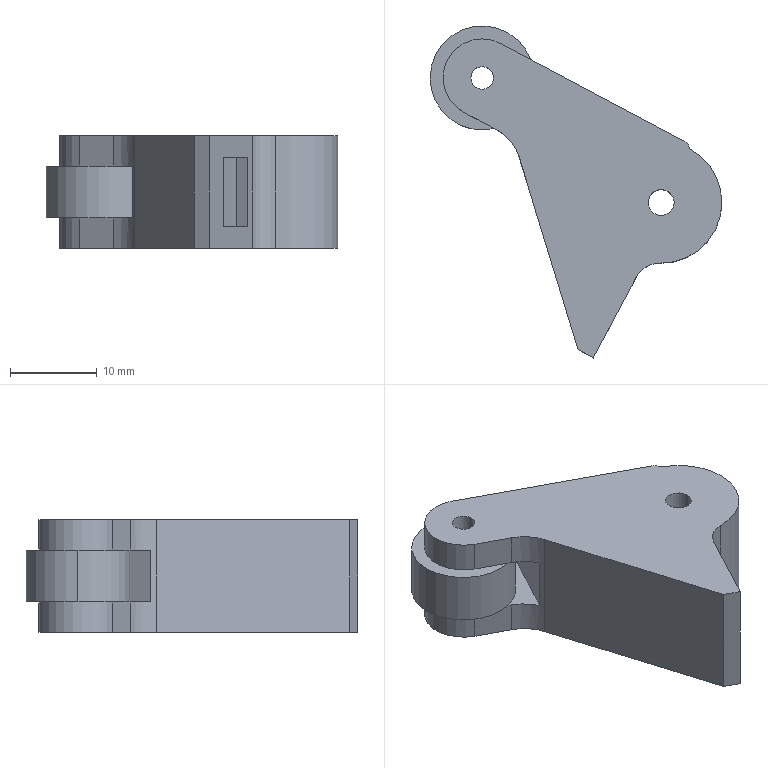Part | STEP file | 1105WWT3_1 | 1 solid | 33 faces | box 33.665 x 38.307 x 13 mm | volume 6665 mm3 | plane 19 | cylinder 14 | commonest cylinder face diameters 2.6 x2 3 x2 9 x2 12 x2 14 x2 1 x1
STEP:
#1=CARTESIAN_POINT('',(-37.5,12.,-6.5));
#2=VERTEX_POINT('',#1);
#3=CARTESIAN_POINT('',(-34.5,12.,-6.5));
#4=VERTEX_POINT('',#3);
#5=CARTESIAN_POINT('',(-36.,12.,-6.5));
#6=DIRECTION('',(0.,0.,1.));
#7=DIRECTION('',(1.,0.,0.));
#8=AXIS2_PLACEMENT_3D('',#5,#6,#7);
#9=CIRCLE('',#8,1.5);
#10=EDGE_CURVE('',#2,#4,#9,.T.);
#11=ORIENTED_EDGE('',*,*,#10,.F.);
#12=CARTESIAN_POINT('',(-37.5,12.,6.5));
#13=VERTEX_POINT('',#12);
#14=CARTESIAN_POINT('',(-37.5,12.,6.5));
#15=DIRECTION('',(0.,0.,1.));
#16=VECTOR('',#15,1000.);
#17=LINE('',#14,#16);
#18=EDGE_CURVE('',#2,#13,#17,.T.);
#19=ORIENTED_EDGE('',*,*,#18,.T.);
#20=CARTESIAN_POINT('',(-34.5,12.,6.5));
#21=VERTEX_POINT('',#20);
#22=CARTESIAN_POINT('',(-36.,12.,6.5));
#23=DIRECTION('',(0.,0.,-1.));
#24=DIRECTION('',(1.,0.,0.));
#25=AXIS2_PLACEMENT_3D('',#22,#23,#24);
#26=CIRCLE('',#25,1.5);
#27=EDGE_CURVE('',#21,#13,#26,.T.);
#28=ORIENTED_EDGE('',*,*,#27,.F.);
#29=CARTESIAN_POINT('',(-34.5,12.,6.5));
#30=DIRECTION('',(0.,0.,1.));
#31=VECTOR('',#30,1000.);
#32=LINE('',#29,#31);
#33=EDGE_CURVE('',#4,#21,#32,.T.);
#34=ORIENTED_EDGE('',*,*,#33,.F.);
#35=EDGE_LOOP('',(#11,#19,#28,#34));
#36=FACE_OUTER_BOUND('',#35,.T.);
#37=CARTESIAN_POINT('',(-36.,12.,6.5));
#38=DIRECTION('',(0.,0.,1.));
#39=DIRECTION('',(1.,0.,0.));
#40=AXIS2_PLACEMENT_3D('',#37,#38,#39);
#41=CYLINDRICAL_SURFACE('',#40,1.5);
#42=ADVANCED_FACE('',(#36),#41,.F.);
#43=CARTESIAN_POINT('',(-57.965,26.386,-6.5));
#44=VERTEX_POINT('',#43);
#45=CARTESIAN_POINT('',(-55.365,26.386,-6.5));
#46=VERTEX_POINT('',#45);
#47=CARTESIAN_POINT('',(-56.665,26.386,-6.5));
#48=DIRECTION('',(0.,0.,1.));
#49=DIRECTION('',(1.,0.,0.));
#50=AXIS2_PLACEMENT_3D('',#47,#48,#49);
#51=CIRCLE('',#50,1.3);
#52=EDGE_CURVE('',#44,#46,#51,.T.);
#53=ORIENTED_EDGE('',*,*,#52,.F.);
#54=CARTESIAN_POINT('',(-57.965,26.386,6.5));
#55=VERTEX_POINT('',#54);
#56=CARTESIAN_POINT('',(-57.965,26.386,6.5));
#57=DIRECTION('',(0.,0.,1.));
#58=VECTOR('',#57,1000.);
#59=LINE('',#56,#58);
#60=EDGE_CURVE('',#44,#55,#59,.T.);
#61=ORIENTED_EDGE('',*,*,#60,.T.);
#62=CARTESIAN_POINT('',(-55.365,26.386,6.5));
#63=VERTEX_POINT('',#62);
#64=CARTESIAN_POINT('',(-56.665,26.386,6.5));
#65=DIRECTION('',(0.,0.,-1.));
#66=DIRECTION('',(1.,0.,0.));
#67=AXIS2_PLACEMENT_3D('',#64,#65,#66);
#68=CIRCLE('',#67,1.3);
#69=EDGE_CURVE('',#63,#55,#68,.T.);
#70=ORIENTED_EDGE('',*,*,#69,.F.);
#71=CARTESIAN_POINT('',(-55.365,26.386,6.5));
#72=DIRECTION('',(0.,0.,1.));
#73=VECTOR('',#72,1000.);
#74=LINE('',#71,#73);
#75=EDGE_CURVE('',#46,#63,#74,.T.);
#76=ORIENTED_EDGE('',*,*,#75,.F.);
#77=EDGE_LOOP('',(#53,#61,#70,#76));
#78=FACE_OUTER_BOUND('',#77,.T.);
#79=CARTESIAN_POINT('',(-56.665,26.386,6.5));
#80=DIRECTION('',(0.,0.,1.));
#81=DIRECTION('',(1.,0.,0.));
#82=AXIS2_PLACEMENT_3D('',#79,#80,#81);
#83=CYLINDRICAL_SURFACE('',#82,1.3);
#84=ADVANCED_FACE('',(#78),#83,.F.);
#85=CARTESIAN_POINT('',(-36.153,5.002,-6.5));
#86=VERTEX_POINT('',#85);
#87=CARTESIAN_POINT('',(-29.,12.,-6.5));
#88=VERTEX_POINT('',#87);
#89=CARTESIAN_POINT('',(-36.,12.,-6.5));
#90=DIRECTION('',(0.,0.,1.));
#91=DIRECTION('',(1.,0.,0.));
#92=AXIS2_PLACEMENT_3D('',#89,#90,#91);
#93=CIRCLE('',#92,7.);
#94=EDGE_CURVE('',#86,#88,#93,.T.);
#95=ORIENTED_EDGE('',*,*,#94,.T.);
#96=CARTESIAN_POINT('',(-29.,12.,6.5));
#97=VERTEX_POINT('',#96);
#98=CARTESIAN_POINT('',(-29.,12.,6.5));
#99=DIRECTION('',(0.,0.,1.));
#100=VECTOR('',#99,1000.);
#101=LINE('',#98,#100);
#102=EDGE_CURVE('',#88,#97,#101,.T.);
#103=ORIENTED_EDGE('',*,*,#102,.T.);
#104=CARTESIAN_POINT('',(-36.153,5.002,6.5));
#105=VERTEX_POINT('',#104);
#106=CARTESIAN_POINT('',(-36.,12.,6.5));
#107=DIRECTION('',(0.,0.,1.));
#108=DIRECTION('',(1.,0.,0.));
#109=AXIS2_PLACEMENT_3D('',#106,#107,#108);
#110=CIRCLE('',#109,7.);
#111=EDGE_CURVE('',#105,#97,#110,.T.);
#112=ORIENTED_EDGE('',*,*,#111,.F.);
#113=CARTESIAN_POINT('',(-36.153,5.002,6.5));
#114=DIRECTION('',(0.,0.,-1.));
#115=VECTOR('',#114,1000.);
#116=LINE('',#113,#115);
#117=EDGE_CURVE('',#105,#86,#116,.T.);
#118=ORIENTED_EDGE('',*,*,#117,.T.);
#119=EDGE_LOOP('',(#95,#103,#112,#118));
#120=FACE_OUTER_BOUND('',#119,.T.);
#121=CARTESIAN_POINT('',(-36.,12.,6.5));
#122=DIRECTION('',(0.,0.,1.));
#123=DIRECTION('',(1.,0.,0.));
#124=AXIS2_PLACEMENT_3D('',#121,#122,#123);
#125=CYLINDRICAL_SURFACE('',#124,7.);
#126=ADVANCED_FACE('',(#120),#125,.T.);
#127=CARTESIAN_POINT('',(-51.049,28.496,-3.));
#128=VERTEX_POINT('',#127);
#129=CARTESIAN_POINT('',(-62.665,26.386,-3.));
#130=VERTEX_POINT('',#129);
#131=CARTESIAN_POINT('',(-56.665,26.386,-3.));
#132=DIRECTION('',(0.,0.,1.));
#133=DIRECTION('',(1.,0.,0.));
#134=AXIS2_PLACEMENT_3D('',#131,#132,#133);
#135=CIRCLE('',#134,6.);
#136=EDGE_CURVE('',#128,#130,#135,.T.);
#137=ORIENTED_EDGE('',*,*,#136,.T.);
#138=CARTESIAN_POINT('',(-62.665,26.386,3.));
#139=VERTEX_POINT('',#138);
#140=CARTESIAN_POINT('',(-62.665,26.386,3.));
#141=DIRECTION('',(0.,0.,1.));
#142=VECTOR('',#141,1000.);
#143=LINE('',#140,#142);
#144=EDGE_CURVE('',#130,#139,#143,.T.);
#145=ORIENTED_EDGE('',*,*,#144,.T.);
#146=CARTESIAN_POINT('',(-51.049,28.496,3.));
#147=VERTEX_POINT('',#146);
#148=CARTESIAN_POINT('',(-56.665,26.386,3.));
#149=DIRECTION('',(0.,0.,1.));
#150=DIRECTION('',(1.,0.,0.));
#151=AXIS2_PLACEMENT_3D('',#148,#149,#150);
#152=CIRCLE('',#151,6.);
#153=EDGE_CURVE('',#147,#139,#152,.T.);
#154=ORIENTED_EDGE('',*,*,#153,.F.);
#155=CARTESIAN_POINT('',(-50.665,26.386,3.));
#156=VERTEX_POINT('',#155);
#157=CARTESIAN_POINT('',(-56.665,26.386,3.));
#158=DIRECTION('',(0.,0.,-1.));
#159=DIRECTION('',(1.,0.,0.));
#160=AXIS2_PLACEMENT_3D('',#157,#158,#159);
#161=CIRCLE('',#160,6.);
#162=EDGE_CURVE('',#147,#156,#161,.T.);
#163=ORIENTED_EDGE('',*,*,#162,.T.);
#164=CARTESIAN_POINT('',(-50.665,26.386,-3.));
#165=VERTEX_POINT('',#164);
#166=CARTESIAN_POINT('',(-50.665,26.386,3.));
#167=DIRECTION('',(0.,0.,1.));
#168=VECTOR('',#167,1000.);
#169=LINE('',#166,#168);
#170=EDGE_CURVE('',#165,#156,#169,.T.);
#171=ORIENTED_EDGE('',*,*,#170,.F.);
#172=CARTESIAN_POINT('',(-56.665,26.386,-3.));
#173=DIRECTION('',(0.,0.,-1.));
#174=DIRECTION('',(1.,0.,0.));
#175=AXIS2_PLACEMENT_3D('',#172,#173,#174);
#176=CIRCLE('',#175,6.);
#177=EDGE_CURVE('',#128,#165,#176,.T.);
#178=ORIENTED_EDGE('',*,*,#177,.F.);
#179=EDGE_LOOP('',(#137,#145,#154,#163,#171,#178));
#180=FACE_OUTER_BOUND('',#179,.T.);
#181=CARTESIAN_POINT('',(-56.665,26.386,3.));
#182=DIRECTION('',(0.,0.,1.));
#183=DIRECTION('',(1.,0.,0.));
#184=AXIS2_PLACEMENT_3D('',#181,#182,#183);
#185=CYLINDRICAL_SURFACE('',#184,6.);
#186=ADVANCED_FACE('',(#180),#185,.T.);
#187=ORIENTED_EDGE('',*,*,#27,.T.);
#188=CARTESIAN_POINT('',(-36.,12.,6.5));
#189=DIRECTION('',(0.,0.,-1.));
#190=DIRECTION('',(1.,0.,0.));
#191=AXIS2_PLACEMENT_3D('',#188,#189,#190);
#192=CIRCLE('',#191,1.5);
#193=EDGE_CURVE('',#13,#21,#192,.T.);
#194=ORIENTED_EDGE('',*,*,#193,.T.);
#195=EDGE_LOOP('',(#187,#194));
#196=FACE_BOUND('',#195,.T.);
#197=ORIENTED_EDGE('',*,*,#69,.T.);
#198=CARTESIAN_POINT('',(-56.665,26.386,6.5));
#199=DIRECTION('',(0.,0.,-1.));
#200=DIRECTION('',(1.,0.,0.));
#201=AXIS2_PLACEMENT_3D('',#198,#199,#200);
#202=CIRCLE('',#201,1.3);
#203=EDGE_CURVE('',#55,#63,#202,.T.);
#204=ORIENTED_EDGE('',*,*,#203,.T.);
#205=EDGE_LOOP('',(#197,#204));
#206=FACE_BOUND('',#205,.T.);
#207=CARTESIAN_POINT('',(-52.433,17.38,6.5));
#208=VERTEX_POINT('',#207);
#209=CARTESIAN_POINT('',(-45.596,-4.983,6.5));
#210=VERTEX_POINT('',#209);
#211=CARTESIAN_POINT('',(-52.433,17.38,6.5));
#212=DIRECTION('',(0.2924,-0.9563,0.));
#213=VECTOR('',#212,1000.);
#214=LINE('',#211,#213);
#215=EDGE_CURVE('',#208,#210,#214,.T.);
#216=ORIENTED_EDGE('',*,*,#215,.T.);
#217=CARTESIAN_POINT('',(-43.83,-5.922,6.5));
#218=VERTEX_POINT('',#217);
#219=CARTESIAN_POINT('',(-45.596,-4.983,6.5));
#220=DIRECTION('',(0.8829,-0.4695,0.));
#221=VECTOR('',#220,1000.);
#222=LINE('',#219,#221);
#223=EDGE_CURVE('',#210,#218,#222,.T.);
#224=ORIENTED_EDGE('',*,*,#223,.T.);
#225=CARTESIAN_POINT('',(-38.868,3.411,6.5));
#226=VERTEX_POINT('',#225);
#227=CARTESIAN_POINT('',(-43.83,-5.922,6.5));
#228=DIRECTION('',(0.4695,0.8829,0.));
#229=VECTOR('',#228,1000.);
#230=LINE('',#227,#229);
#231=EDGE_CURVE('',#218,#226,#230,.T.);
#232=ORIENTED_EDGE('',*,*,#231,.T.);
#233=CARTESIAN_POINT('',(-36.219,2.002,6.5));
#234=DIRECTION('',(0.,0.,-1.));
#235=DIRECTION('',(1.,0.,0.));
#236=AXIS2_PLACEMENT_3D('',#233,#234,#235);
#237=CIRCLE('',#236,3.);
#238=EDGE_CURVE('',#226,#105,#237,.T.);
#239=ORIENTED_EDGE('',*,*,#238,.T.);
#240=ORIENTED_EDGE('',*,*,#111,.T.);
#241=CARTESIAN_POINT('',(-32.542,18.086,6.5));
#242=VERTEX_POINT('',#241);
#243=CARTESIAN_POINT('',(-36.,12.,6.5));
#244=DIRECTION('',(0.,0.,1.));
#245=DIRECTION('',(1.,0.,0.));
#246=AXIS2_PLACEMENT_3D('',#243,#244,#245);
#247=CIRCLE('',#246,7.);
#248=EDGE_CURVE('',#97,#242,#247,.T.);
#249=ORIENTED_EDGE('',*,*,#248,.T.);
#250=CARTESIAN_POINT('',(-32.773,18.375,6.5));
#251=VERTEX_POINT('',#250);
#252=CARTESIAN_POINT('',(-32.295,18.521,6.5));
#253=DIRECTION('',(0.,0.,-1.));
#254=DIRECTION('',(1.,0.,0.));
#255=AXIS2_PLACEMENT_3D('',#252,#253,#254);
#256=CIRCLE('',#255,0.5);
#257=EDGE_CURVE('',#242,#251,#256,.T.);
#258=ORIENTED_EDGE('',*,*,#257,.T.);
#259=CARTESIAN_POINT('',(-32.799,18.461,6.5));
#260=VERTEX_POINT('',#259);
#261=CARTESIAN_POINT('',(-32.773,18.375,6.5));
#262=DIRECTION('',(0.2924,-0.9563,0.));
#263=VECTOR('',#262,1000.);
#264=LINE('',#261,#263);
#265=EDGE_CURVE('',#260,#251,#264,.T.);
#266=ORIENTED_EDGE('',*,*,#265,.F.);
#267=CARTESIAN_POINT('',(-33.286,19.051,6.5));
#268=VERTEX_POINT('',#267);
#269=CARTESIAN_POINT('',(-33.756,18.168,6.5));
#270=DIRECTION('',(0.,0.,-1.));
#271=DIRECTION('',(1.,0.,0.));
#272=AXIS2_PLACEMENT_3D('',#269,#270,#271);
#273=CIRCLE('',#272,1.);
#274=EDGE_CURVE('',#268,#260,#273,.T.);
#275=ORIENTED_EDGE('',*,*,#274,.F.);
#276=CARTESIAN_POINT('',(-54.553,30.359,6.5));
#277=VERTEX_POINT('',#276);
#278=CARTESIAN_POINT('',(-33.286,19.051,6.5));
#279=DIRECTION('',(-0.8829,0.4695,0.));
#280=VECTOR('',#279,1000.);
#281=LINE('',#278,#280);
#282=EDGE_CURVE('',#268,#277,#281,.T.);
#283=ORIENTED_EDGE('',*,*,#282,.T.);
#284=CARTESIAN_POINT('',(-58.778,22.412,6.5));
#285=VERTEX_POINT('',#284);
#286=CARTESIAN_POINT('',(-56.665,26.386,6.5));
#287=DIRECTION('',(0.,0.,1.));
#288=DIRECTION('',(1.,0.,0.));
#289=AXIS2_PLACEMENT_3D('',#286,#287,#288);
#290=CIRCLE('',#289,4.5);
#291=EDGE_CURVE('',#277,#285,#290,.T.);
#292=ORIENTED_EDGE('',*,*,#291,.T.);
#293=CARTESIAN_POINT('',(-54.867,20.333,6.5));
#294=VERTEX_POINT('',#293);
#295=CARTESIAN_POINT('',(-58.778,22.412,6.5));
#296=DIRECTION('',(0.8829,-0.4695,0.));
#297=VECTOR('',#296,1000.);
#298=LINE('',#295,#297);
#299=EDGE_CURVE('',#285,#294,#298,.T.);
#300=ORIENTED_EDGE('',*,*,#299,.T.);
#301=CARTESIAN_POINT('',(-57.215,15.918,6.5));
#302=DIRECTION('',(0.,0.,-1.));
#303=DIRECTION('',(1.,0.,0.));
#304=AXIS2_PLACEMENT_3D('',#301,#302,#303);
#305=CIRCLE('',#304,5.);
#306=EDGE_CURVE('',#294,#208,#305,.T.);
#307=ORIENTED_EDGE('',*,*,#306,.T.);
#308=EDGE_LOOP('',(#216,#224,#232,#239,#240,#249,#258,#266,#275,#283,#292,#300,#307));
#309=FACE_OUTER_BOUND('',#308,.T.);
#310=CARTESIAN_POINT('',(-36.,12.,6.5));
#311=DIRECTION('',(0.,0.,1.));
#312=DIRECTION('',(1.,0.,0.));
#313=AXIS2_PLACEMENT_3D('',#310,#311,#312);
#314=PLANE('',#313);
#315=ADVANCED_FACE('',(#196,#206,#309),#314,.T.);
#316=ORIENTED_EDGE('',*,*,#18,.F.);
#317=CARTESIAN_POINT('',(-36.,12.,-6.5));
#318=DIRECTION('',(0.,0.,1.));
#319=DIRECTION('',(1.,0.,0.));
#320=AXIS2_PLACEMENT_3D('',#317,#318,#319);
#321=CIRCLE('',#320,1.5);
#322=EDGE_CURVE('',#4,#2,#321,.T.);
#323=ORIENTED_EDGE('',*,*,#322,.F.);
#324=ORIENTED_EDGE('',*,*,#33,.T.);
#325=ORIENTED_EDGE('',*,*,#193,.F.);
#326=EDGE_LOOP('',(#316,#323,#324,#325));
#327=FACE_OUTER_BOUND('',#326,.T.);
#328=CARTESIAN_POINT('',(-36.,12.,6.5));
#329=DIRECTION('',(0.,0.,1.));
#330=DIRECTION('',(1.,0.,0.));
#331=AXIS2_PLACEMENT_3D('',#328,#329,#330);
#332=CYLINDRICAL_SURFACE('',#331,1.5);
#333=ADVANCED_FACE('',(#327),#332,.F.);
#334=ORIENTED_EDGE('',*,*,#60,.F.);
#335=CARTESIAN_POINT('',(-56.665,26.386,-6.5));
#336=DIRECTION('',(0.,0.,1.));
#337=DIRECTION('',(1.,0.,0.));
#338=AXIS2_PLACEMENT_3D('',#335,#336,#337);
#339=CIRCLE('',#338,1.3);
#340=EDGE_CURVE('',#46,#44,#339,.T.);
#341=ORIENTED_EDGE('',*,*,#340,.F.);
#342=ORIENTED_EDGE('',*,*,#75,.T.);
#343=ORIENTED_EDGE('',*,*,#203,.F.);
#344=EDGE_LOOP('',(#334,#341,#342,#343));
#345=FACE_OUTER_BOUND('',#344,.T.);
#346=CARTESIAN_POINT('',(-56.665,26.386,6.5));
#347=DIRECTION('',(0.,0.,1.));
#348=DIRECTION('',(1.,0.,0.));
#349=AXIS2_PLACEMENT_3D('',#346,#347,#348);
#350=CYLINDRICAL_SURFACE('',#349,1.3);
#351=ADVANCED_FACE('',(#345),#350,.F.);
#352=ORIENTED_EDGE('',*,*,#223,.F.);
#353=CARTESIAN_POINT('',(-45.596,-4.983,-6.5));
#354=VERTEX_POINT('',#353);
#355=CARTESIAN_POINT('',(-45.596,-4.983,6.5));
#356=DIRECTION('',(0.,0.,-1.));
#357=VECTOR('',#356,1000.);
#358=LINE('',#355,#357);
#359=EDGE_CURVE('',#210,#354,#358,.T.);
#360=ORIENTED_EDGE('',*,*,#359,.T.);
#361=CARTESIAN_POINT('',(-43.83,-5.922,-6.5));
#362=VERTEX_POINT('',#361);
#363=CARTESIAN_POINT('',(-45.596,-4.983,-6.5));
#364=DIRECTION('',(0.8829,-0.4695,0.));
#365=VECTOR('',#364,1000.);
#366=LINE('',#363,#365);
#367=EDGE_CURVE('',#354,#362,#366,.T.);
#368=ORIENTED_EDGE('',*,*,#367,.T.);
#369=CARTESIAN_POINT('',(-43.83,-5.922,6.5));
#370=DIRECTION('',(0.,0.,1.));
#371=VECTOR('',#370,1000.);
#372=LINE('',#369,#371);
#373=EDGE_CURVE('',#362,#218,#372,.T.);
#374=ORIENTED_EDGE('',*,*,#373,.T.);
#375=EDGE_LOOP('',(#352,#360,#368,#374));
#376=FACE_OUTER_BOUND('',#375,.T.);
#377=CARTESIAN_POINT('',(-45.596,-4.983,6.5));
#378=DIRECTION('',(-0.4695,-0.8829,0.));
#379=DIRECTION('',(0.8829,-0.4695,0.));
#380=AXIS2_PLACEMENT_3D('',#377,#378,#379);
#381=PLANE('',#380);
#382=ADVANCED_FACE('',(#376),#381,.T.);
#383=ORIENTED_EDGE('',*,*,#215,.F.);
#384=CARTESIAN_POINT('',(-52.433,17.38,-6.5));
#385=VERTEX_POINT('',#384);
#386=CARTESIAN_POINT('',(-52.433,17.38,6.5));
#387=DIRECTION('',(0.,0.,-1.));
#388=VECTOR('',#387,1000.);
#389=LINE('',#386,#388);
#390=EDGE_CURVE('',#208,#385,#389,.T.);
#391=ORIENTED_EDGE('',*,*,#390,.T.);
#392=CARTESIAN_POINT('',(-52.433,17.38,-6.5));
#393=DIRECTION('',(0.2924,-0.9563,0.));
#394=VECTOR('',#393,1000.);
#395=LINE('',#392,#394);
#396=EDGE_CURVE('',#385,#354,#395,.T.);
#397=ORIENTED_EDGE('',*,*,#396,.T.);
#398=ORIENTED_EDGE('',*,*,#359,.F.);
#399=EDGE_LOOP('',(#383,#391,#397,#398));
#400=FACE_OUTER_BOUND('',#399,.T.);
#401=CARTESIAN_POINT('',(-52.433,17.38,6.5));
#402=DIRECTION('',(-0.9563,-0.2924,0.));
#403=DIRECTION('',(0.2924,-0.9563,0.));
#404=AXIS2_PLACEMENT_3D('',#401,#402,#403);
#405=PLANE('',#404);
#406=ADVANCED_FACE('',(#400),#405,.T.);
#407=CARTESIAN_POINT('',(-54.867,20.333,-6.5));
#408=VERTEX_POINT('',#407);
#409=CARTESIAN_POINT('',(-54.867,20.333,-3.));
#410=VERTEX_POINT('',#409);
#411=CARTESIAN_POINT('',(-54.867,20.333,6.5));
#412=DIRECTION('',(0.,0.,1.));
#413=VECTOR('',#412,1000.);
#414=LINE('',#411,#413);
#415=EDGE_CURVE('',#408,#410,#414,.T.);
#416=ORIENTED_EDGE('',*,*,#415,.F.);
#417=CARTESIAN_POINT('',(-57.215,15.918,-6.5));
#418=DIRECTION('',(0.,0.,1.));
#419=DIRECTION('',(1.,0.,0.));
#420=AXIS2_PLACEMENT_3D('',#417,#418,#419);
#421=CIRCLE('',#420,5.);
#422=EDGE_CURVE('',#385,#408,#421,.T.);
#423=ORIENTED_EDGE('',*,*,#422,.F.);
#424=ORIENTED_EDGE('',*,*,#390,.F.);
#425=ORIENTED_EDGE('',*,*,#306,.F.);
#426=CARTESIAN_POINT('',(-54.867,20.333,3.));
#427=VERTEX_POINT('',#426);
#428=CARTESIAN_POINT('',(-54.867,20.333,6.5));
#429=DIRECTION('',(0.,0.,1.));
#430=VECTOR('',#429,1000.);
#431=LINE('',#428,#430);
#432=EDGE_CURVE('',#427,#294,#431,.T.);
#433=ORIENTED_EDGE('',*,*,#432,.F.);
#434=CARTESIAN_POINT('',(-52.651,17.96,3.));
#435=VERTEX_POINT('',#434);
#436=CARTESIAN_POINT('',(-57.215,15.918,3.));
#437=DIRECTION('',(0.,0.,1.));
#438=DIRECTION('',(1.,0.,0.));
#439=AXIS2_PLACEMENT_3D('',#436,#437,#438);
#440=CIRCLE('',#439,5.);
#441=EDGE_CURVE('',#435,#427,#440,.T.);
#442=ORIENTED_EDGE('',*,*,#441,.F.);
#443=CARTESIAN_POINT('',(-52.651,17.96,-3.));
#444=VERTEX_POINT('',#443);
#445=CARTESIAN_POINT('',(-52.651,17.96,6.5));
#446=DIRECTION('',(0.,0.,1.));
#447=VECTOR('',#446,1000.);
#448=LINE('',#445,#447);
#449=EDGE_CURVE('',#444,#435,#448,.T.);
#450=ORIENTED_EDGE('',*,*,#449,.F.);
#451=CARTESIAN_POINT('',(-57.215,15.918,-3.));
#452=DIRECTION('',(0.,0.,-1.));
#453=DIRECTION('',(1.,0.,0.));
#454=AXIS2_PLACEMENT_3D('',#451,#452,#453);
#455=CIRCLE('',#454,5.);
#456=EDGE_CURVE('',#410,#444,#455,.T.);
#457=ORIENTED_EDGE('',*,*,#456,.F.);
#458=EDGE_LOOP('',(#416,#423,#424,#425,#433,#442,#450,#457));
#459=FACE_OUTER_BOUND('',#458,.T.);
#460=CARTESIAN_POINT('',(-57.215,15.918,6.5));
#461=DIRECTION('',(0.,0.,1.));
#462=DIRECTION('',(1.,0.,0.));
#463=AXIS2_PLACEMENT_3D('',#460,#461,#462);
#464=CYLINDRICAL_SURFACE('',#463,5.);
#465=ADVANCED_FACE('',(#459),#464,.F.);
#466=ORIENTED_EDGE('',*,*,#299,.F.);
#467=CARTESIAN_POINT('',(-58.778,22.412,3.));
#468=VERTEX_POINT('',#467);
#469=CARTESIAN_POINT('',(-58.778,22.412,6.5));
#470=DIRECTION('',(0.,0.,-1.));
#471=VECTOR('',#470,1000.);
#472=LINE('',#469,#471);
#473=EDGE_CURVE('',#285,#468,#472,.T.);
#474=ORIENTED_EDGE('',*,*,#473,.T.);
#475=CARTESIAN_POINT('',(-55.274,20.549,3.));
#476=VERTEX_POINT('',#475);
#477=CARTESIAN_POINT('',(-58.778,22.412,3.));
#478=DIRECTION('',(0.8829,-0.4695,0.));
#479=VECTOR('',#478,1000.);
#480=LINE('',#477,#479);
#481=EDGE_CURVE('',#468,#476,#480,.T.);
#482=ORIENTED_EDGE('',*,*,#481,.T.);
#483=CARTESIAN_POINT('',(-58.778,22.412,3.));
#484=DIRECTION('',(0.8829,-0.4695,0.));
#485=VECTOR('',#484,1000.);
#486=LINE('',#483,#485);
#487=EDGE_CURVE('',#476,#427,#486,.T.);
#488=ORIENTED_EDGE('',*,*,#487,.T.);
#489=ORIENTED_EDGE('',*,*,#432,.T.);
#490=EDGE_LOOP('',(#466,#474,#482,#488,#489));
#491=FACE_OUTER_BOUND('',#490,.T.);
#492=CARTESIAN_POINT('',(-58.778,22.412,6.5));
#493=DIRECTION('',(-0.4695,-0.8829,0.));
#494=DIRECTION('',(0.8829,-0.4695,0.));
#495=AXIS2_PLACEMENT_3D('',#492,#493,#494);
#496=PLANE('',#495);
#497=ADVANCED_FACE('',(#491),#496,.T.);
#498=ORIENTED_EDGE('',*,*,#291,.F.);
#499=CARTESIAN_POINT('',(-54.553,30.359,3.));
#500=VERTEX_POINT('',#499);
#501=CARTESIAN_POINT('',(-54.553,30.359,6.5));
#502=DIRECTION('',(0.,0.,-1.));
#503=VECTOR('',#502,1000.);
#504=LINE('',#501,#503);
#505=EDGE_CURVE('',#277,#500,#504,.T.);
#506=ORIENTED_EDGE('',*,*,#505,.T.);
#507=CARTESIAN_POINT('',(-56.665,26.386,3.));
#508=DIRECTION('',(0.,0.,1.));
#509=DIRECTION('',(1.,0.,0.));
#510=AXIS2_PLACEMENT_3D('',#507,#508,#509);
#511=CIRCLE('',#510,4.5);
#512=EDGE_CURVE('',#500,#468,#511,.T.);
#513=ORIENTED_EDGE('',*,*,#512,.T.);
#514=ORIENTED_EDGE('',*,*,#473,.F.);
#515=EDGE_LOOP('',(#498,#506,#513,#514));
#516=FACE_OUTER_BOUND('',#515,.T.);
#517=CARTESIAN_POINT('',(-56.665,26.386,6.5));
#518=DIRECTION('',(0.,0.,1.));
#519=DIRECTION('',(1.,0.,0.));
#520=AXIS2_PLACEMENT_3D('',#517,#518,#519);
#521=CYLINDRICAL_SURFACE('',#520,4.5);
#522=ADVANCED_FACE('',(#516),#521,.T.);
#523=CARTESIAN_POINT('',(-33.286,19.051,-6.5));
#524=VERTEX_POINT('',#523);
#525=CARTESIAN_POINT('',(-54.553,30.359,-6.5));
#526=VERTEX_POINT('',#525);
#527=CARTESIAN_POINT('',(-33.286,19.051,-6.5));
#528=DIRECTION('',(-0.8829,0.4695,0.));
#529=VECTOR('',#528,1000.);
#530=LINE('',#527,#529);
#531=EDGE_CURVE('',#524,#526,#530,.T.);
#532=ORIENTED_EDGE('',*,*,#531,.T.);
#533=CARTESIAN_POINT('',(-54.553,30.359,-3.));
#534=VERTEX_POINT('',#533);
#535=CARTESIAN_POINT('',(-54.553,30.359,6.5));
#536=DIRECTION('',(0.,0.,1.));
#537=VECTOR('',#536,1000.);
#538=LINE('',#535,#537);
#539=EDGE_CURVE('',#526,#534,#538,.T.);
#540=ORIENTED_EDGE('',*,*,#539,.T.);
#541=CARTESIAN_POINT('',(-33.286,19.051,-3.));
#542=DIRECTION('',(0.8829,-0.4695,0.));
#543=VECTOR('',#542,1000.);
#544=LINE('',#541,#543);
#545=EDGE_CURVE('',#534,#128,#544,.T.);
#546=ORIENTED_EDGE('',*,*,#545,.T.);
#547=CARTESIAN_POINT('',(-47.931,26.838,-3.));
#548=VERTEX_POINT('',#547);
#549=CARTESIAN_POINT('',(-33.286,19.051,-3.));
#550=DIRECTION('',(0.8829,-0.4695,0.));
#551=VECTOR('',#550,1000.);
#552=LINE('',#549,#551);
#553=EDGE_CURVE('',#128,#548,#552,.T.);
#554=ORIENTED_EDGE('',*,*,#553,.T.);
#555=CARTESIAN_POINT('',(-47.931,26.838,3.));
#556=VERTEX_POINT('',#555);
#557=CARTESIAN_POINT('',(-47.931,26.838,6.5));
#558=DIRECTION('',(0.,0.,1.));
#559=VECTOR('',#558,1000.);
#560=LINE('',#557,#559);
#561=EDGE_CURVE('',#548,#556,#560,.T.);
#562=ORIENTED_EDGE('',*,*,#561,.T.);
#563=CARTESIAN_POINT('',(-33.286,19.051,3.));
#564=DIRECTION('',(-0.8829,0.4695,0.));
#565=VECTOR('',#564,1000.);
#566=LINE('',#563,#565);
#567=EDGE_CURVE('',#556,#147,#566,.T.);
#568=ORIENTED_EDGE('',*,*,#567,.T.);
#569=CARTESIAN_POINT('',(-33.286,19.051,3.));
#570=DIRECTION('',(-0.8829,0.4695,0.));
#571=VECTOR('',#570,1000.);
#572=LINE('',#569,#571);
#573=EDGE_CURVE('',#147,#500,#572,.T.);
#574=ORIENTED_EDGE('',*,*,#573,.T.);
#575=ORIENTED_EDGE('',*,*,#505,.F.);
#576=ORIENTED_EDGE('',*,*,#282,.F.);
#577=CARTESIAN_POINT('',(-33.286,19.051,6.5));
#578=DIRECTION('',(0.,0.,-1.));
#579=VECTOR('',#578,1000.);
#580=LINE('',#577,#579);
#581=EDGE_CURVE('',#268,#524,#580,.T.);
#582=ORIENTED_EDGE('',*,*,#581,.T.);
#583=EDGE_LOOP('',(#532,#540,#546,#554,#562,#568,#574,#575,#576,#582));
#584=FACE_OUTER_BOUND('',#583,.T.);
#585=CARTESIAN_POINT('',(-33.286,19.051,6.5));
#586=DIRECTION('',(0.4695,0.8829,0.));
#587=DIRECTION('',(-0.8829,0.4695,0.));
#588=AXIS2_PLACEMENT_3D('',#585,#586,#587);
#589=PLANE('',#588);
#590=ADVANCED_FACE('',(#584),#589,.T.);
#591=ORIENTED_EDGE('',*,*,#102,.F.);
#592=CARTESIAN_POINT('',(-32.542,18.086,-6.5));
#593=VERTEX_POINT('',#592);
#594=CARTESIAN_POINT('',(-36.,12.,-6.5));
#595=DIRECTION('',(0.,0.,1.));
#596=DIRECTION('',(1.,0.,0.));
#597=AXIS2_PLACEMENT_3D('',#594,#595,#596);
#598=CIRCLE('',#597,7.);
#599=EDGE_CURVE('',#88,#593,#598,.T.);
#600=ORIENTED_EDGE('',*,*,#599,.T.);
#601=CARTESIAN_POINT('',(-32.542,18.086,6.5));
#602=DIRECTION('',(0.,0.,1.));
#603=VECTOR('',#602,1000.);
#604=LINE('',#601,#603);
#605=EDGE_CURVE('',#593,#242,#604,.T.);
#606=ORIENTED_EDGE('',*,*,#605,.T.);
#607=ORIENTED_EDGE('',*,*,#248,.F.);
#608=EDGE_LOOP('',(#591,#600,#606,#607));
#609=FACE_OUTER_BOUND('',#608,.T.);
#610=CARTESIAN_POINT('',(-36.,12.,6.5));
#611=DIRECTION('',(0.,0.,1.));
#612=DIRECTION('',(1.,0.,0.));
#613=AXIS2_PLACEMENT_3D('',#610,#611,#612);
#614=CYLINDRICAL_SURFACE('',#613,7.);
#615=ADVANCED_FACE('',(#609),#614,.T.);
#616=ORIENTED_EDGE('',*,*,#117,.F.);
#617=ORIENTED_EDGE('',*,*,#238,.F.);
#618=CARTESIAN_POINT('',(-38.868,3.411,-6.5));
#619=VERTEX_POINT('',#618);
#620=CARTESIAN_POINT('',(-38.868,3.411,6.5));
#621=DIRECTION('',(0.,0.,1.));
#622=VECTOR('',#621,1000.);
#623=LINE('',#620,#622);
#624=EDGE_CURVE('',#619,#226,#623,.T.);
#625=ORIENTED_EDGE('',*,*,#624,.F.);
#626=CARTESIAN_POINT('',(-36.219,2.002,-6.5));
#627=DIRECTION('',(0.,0.,1.));
#628=DIRECTION('',(1.,0.,0.));
#629=AXIS2_PLACEMENT_3D('',#626,#627,#628);
#630=CIRCLE('',#629,3.);
#631=EDGE_CURVE('',#86,#619,#630,.T.);
#632=ORIENTED_EDGE('',*,*,#631,.F.);
#633=EDGE_LOOP('',(#616,#617,#625,#632));
#634=FACE_OUTER_BOUND('',#633,.T.);
#635=CARTESIAN_POINT('',(-36.219,2.002,6.5));
#636=DIRECTION('',(0.,0.,1.));
#637=DIRECTION('',(1.,0.,0.));
#638=AXIS2_PLACEMENT_3D('',#635,#636,#637);
#639=CYLINDRICAL_SURFACE('',#638,3.);
#640=ADVANCED_FACE('',(#634),#639,.F.);
#641=ORIENTED_EDGE('',*,*,#231,.F.);
#642=ORIENTED_EDGE('',*,*,#373,.F.);
#643=CARTESIAN_POINT('',(-43.83,-5.922,-6.5));
#644=DIRECTION('',(0.4695,0.8829,0.));
#645=VECTOR('',#644,1000.);
#646=LINE('',#643,#645);
#647=EDGE_CURVE('',#362,#619,#646,.T.);
#648=ORIENTED_EDGE('',*,*,#647,.T.);
#649=ORIENTED_EDGE('',*,*,#624,.T.);
#650=EDGE_LOOP('',(#641,#642,#648,#649));
#651=FACE_OUTER_BOUND('',#650,.T.);
#652=CARTESIAN_POINT('',(-39.37,2.466,4.));
#653=VERTEX_POINT('',#652);
#654=CARTESIAN_POINT('',(-39.37,2.466,-4.));
#655=VERTEX_POINT('',#654);
#656=CARTESIAN_POINT('',(-39.37,2.466,6.5));
#657=DIRECTION('',(0.,0.,-1.));
#658=VECTOR('',#657,1000.);
#659=LINE('',#656,#658);
#660=EDGE_CURVE('',#653,#655,#659,.T.);
#661=ORIENTED_EDGE('',*,*,#660,.T.);
#662=CARTESIAN_POINT('',(-42.187,-2.831,-4.));
#663=VERTEX_POINT('',#662);
#664=CARTESIAN_POINT('',(-43.83,-5.922,-4.));
#665=DIRECTION('',(-0.4695,-0.8829,0.));
#666=VECTOR('',#665,1000.);
#667=LINE('',#664,#666);
#668=EDGE_CURVE('',#655,#663,#667,.T.);
#669=ORIENTED_EDGE('',*,*,#668,.T.);
#670=CARTESIAN_POINT('',(-42.187,-2.831,4.));
#671=VERTEX_POINT('',#670);
#672=CARTESIAN_POINT('',(-42.187,-2.831,6.5));
#673=DIRECTION('',(0.,0.,1.));
#674=VECTOR('',#673,1000.);
#675=LINE('',#672,#674);
#676=EDGE_CURVE('',#663,#671,#675,.T.);
#677=ORIENTED_EDGE('',*,*,#676,.T.);
#678=CARTESIAN_POINT('',(-43.83,-5.922,4.));
#679=DIRECTION('',(0.4695,0.8829,0.));
#680=VECTOR('',#679,1000.);
#681=LINE('',#678,#680);
#682=EDGE_CURVE('',#671,#653,#681,.T.);
#683=ORIENTED_EDGE('',*,*,#682,.T.);
#684=EDGE_LOOP('',(#661,#669,#677,#683));
#685=FACE_BOUND('',#684,.T.);
#686=CARTESIAN_POINT('',(-43.83,-5.922,6.5));
#687=DIRECTION('',(0.8829,-0.4695,0.));
#688=DIRECTION('',(0.4695,0.8829,0.));
#689=AXIS2_PLACEMENT_3D('',#686,#687,#688);
#690=PLANE('',#689);
#691=ADVANCED_FACE('',(#651,#685),#690,.T.);
#692=ORIENTED_EDGE('',*,*,#322,.T.);
#693=ORIENTED_EDGE('',*,*,#10,.T.);
#694=EDGE_LOOP('',(#692,#693));
#695=FACE_BOUND('',#694,.T.);
#696=ORIENTED_EDGE('',*,*,#340,.T.);
#697=ORIENTED_EDGE('',*,*,#52,.T.);
#698=EDGE_LOOP('',(#696,#697));
#699=FACE_BOUND('',#698,.T.);
#700=ORIENTED_EDGE('',*,*,#647,.F.);
#701=ORIENTED_EDGE('',*,*,#367,.F.);
#702=ORIENTED_EDGE('',*,*,#396,.F.);
#703=ORIENTED_EDGE('',*,*,#422,.T.);
#704=CARTESIAN_POINT('',(-58.778,22.412,-6.5));
#705=VERTEX_POINT('',#704);
#706=CARTESIAN_POINT('',(-58.778,22.412,-6.5));
#707=DIRECTION('',(0.8829,-0.4695,0.));
#708=VECTOR('',#707,1000.);
#709=LINE('',#706,#708);
#710=EDGE_CURVE('',#705,#408,#709,.T.);
#711=ORIENTED_EDGE('',*,*,#710,.F.);
#712=CARTESIAN_POINT('',(-56.665,26.386,-6.5));
#713=DIRECTION('',(0.,0.,1.));
#714=DIRECTION('',(1.,0.,0.));
#715=AXIS2_PLACEMENT_3D('',#712,#713,#714);
#716=CIRCLE('',#715,4.5);
#717=EDGE_CURVE('',#526,#705,#716,.T.);
#718=ORIENTED_EDGE('',*,*,#717,.F.);
#719=ORIENTED_EDGE('',*,*,#531,.F.);
#720=CARTESIAN_POINT('',(-32.799,18.461,-6.5));
#721=VERTEX_POINT('',#720);
#722=CARTESIAN_POINT('',(-33.756,18.168,-6.5));
#723=DIRECTION('',(0.,0.,1.));
#724=DIRECTION('',(1.,0.,0.));
#725=AXIS2_PLACEMENT_3D('',#722,#723,#724);
#726=CIRCLE('',#725,1.);
#727=EDGE_CURVE('',#721,#524,#726,.T.);
#728=ORIENTED_EDGE('',*,*,#727,.F.);
#729=CARTESIAN_POINT('',(-32.773,18.375,-6.5));
#730=VERTEX_POINT('',#729);
#731=CARTESIAN_POINT('',(-32.773,18.375,-6.5));
#732=DIRECTION('',(-0.2924,0.9563,0.));
#733=VECTOR('',#732,1000.);
#734=LINE('',#731,#733);
#735=EDGE_CURVE('',#730,#721,#734,.T.);
#736=ORIENTED_EDGE('',*,*,#735,.F.);
#737=CARTESIAN_POINT('',(-32.295,18.521,-6.5));
#738=DIRECTION('',(0.,0.,-1.));
#739=DIRECTION('',(1.,0.,0.));
#740=AXIS2_PLACEMENT_3D('',#737,#738,#739);
#741=CIRCLE('',#740,0.5);
#742=EDGE_CURVE('',#593,#730,#741,.T.);
#743=ORIENTED_EDGE('',*,*,#742,.F.);
#744=ORIENTED_EDGE('',*,*,#599,.F.);
#745=ORIENTED_EDGE('',*,*,#94,.F.);
#746=ORIENTED_EDGE('',*,*,#631,.T.);
#747=EDGE_LOOP('',(#700,#701,#702,#703,#711,#718,#719,#728,#736,#743,#744,#745,#746));
#748=FACE_OUTER_BOUND('',#747,.T.);
#749=CARTESIAN_POINT('',(-36.,12.,-6.5));
#750=DIRECTION('',(0.,0.,1.));
#751=DIRECTION('',(1.,0.,0.));
#752=AXIS2_PLACEMENT_3D('',#749,#750,#751);
#753=PLANE('',#752);
#754=ADVANCED_FACE('',(#695,#699,#748),#753,.F.);
#755=CARTESIAN_POINT('',(-52.651,17.96,-3.));
#756=DIRECTION('',(0.4695,0.8829,0.));
#757=VECTOR('',#756,1000.);
#758=LINE('',#755,#757);
#759=EDGE_CURVE('',#444,#548,#758,.T.);
#760=ORIENTED_EDGE('',*,*,#759,.T.);
#761=ORIENTED_EDGE('',*,*,#553,.F.);
#762=ORIENTED_EDGE('',*,*,#177,.T.);
#763=CARTESIAN_POINT('',(-55.274,20.549,-3.));
#764=VERTEX_POINT('',#763);
#765=CARTESIAN_POINT('',(-56.665,26.386,-3.));
#766=DIRECTION('',(0.,0.,-1.));
#767=DIRECTION('',(1.,0.,0.));
#768=AXIS2_PLACEMENT_3D('',#765,#766,#767);
#769=CIRCLE('',#768,6.);
#770=EDGE_CURVE('',#165,#764,#769,.T.);
#771=ORIENTED_EDGE('',*,*,#770,.T.);
#772=CARTESIAN_POINT('',(-55.274,20.549,-3.));
#773=DIRECTION('',(0.8829,-0.4695,0.));
#774=VECTOR('',#773,1000.);
#775=LINE('',#772,#774);
#776=EDGE_CURVE('',#764,#410,#775,.T.);
#777=ORIENTED_EDGE('',*,*,#776,.T.);
#778=ORIENTED_EDGE('',*,*,#456,.T.);
#779=EDGE_LOOP('',(#760,#761,#762,#771,#777,#778));
#780=FACE_OUTER_BOUND('',#779,.T.);
#781=CARTESIAN_POINT('',(-36.,12.,-3.));
#782=DIRECTION('',(0.,0.,1.));
#783=DIRECTION('',(1.,0.,0.));
#784=AXIS2_PLACEMENT_3D('',#781,#782,#783);
#785=PLANE('',#784);
#786=ADVANCED_FACE('',(#780),#785,.T.);
#787=ORIENTED_EDGE('',*,*,#710,.T.);
#788=ORIENTED_EDGE('',*,*,#415,.T.);
#789=ORIENTED_EDGE('',*,*,#776,.F.);
#790=CARTESIAN_POINT('',(-58.778,22.412,-3.));
#791=VERTEX_POINT('',#790);
#792=CARTESIAN_POINT('',(-58.778,22.412,-3.));
#793=DIRECTION('',(-0.8829,0.4695,0.));
#794=VECTOR('',#793,1000.);
#795=LINE('',#792,#794);
#796=EDGE_CURVE('',#764,#791,#795,.T.);
#797=ORIENTED_EDGE('',*,*,#796,.T.);
#798=CARTESIAN_POINT('',(-58.778,22.412,6.5));
#799=DIRECTION('',(0.,0.,-1.));
#800=VECTOR('',#799,1000.);
#801=LINE('',#798,#800);
#802=EDGE_CURVE('',#791,#705,#801,.T.);
#803=ORIENTED_EDGE('',*,*,#802,.T.);
#804=EDGE_LOOP('',(#787,#788,#789,#797,#803));
#805=FACE_OUTER_BOUND('',#804,.T.);
#806=CARTESIAN_POINT('',(-58.778,22.412,6.5));
#807=DIRECTION('',(-0.4695,-0.8829,0.));
#808=DIRECTION('',(0.8829,-0.4695,0.));
#809=AXIS2_PLACEMENT_3D('',#806,#807,#808);
#810=PLANE('',#809);
#811=ADVANCED_FACE('',(#805),#810,.T.);
#812=ORIENTED_EDGE('',*,*,#567,.F.);
#813=CARTESIAN_POINT('',(-52.651,17.96,3.));
#814=DIRECTION('',(0.4695,0.8829,0.));
#815=VECTOR('',#814,1000.);
#816=LINE('',#813,#815);
#817=EDGE_CURVE('',#435,#556,#816,.T.);
#818=ORIENTED_EDGE('',*,*,#817,.F.);
#819=ORIENTED_EDGE('',*,*,#441,.T.);
#820=ORIENTED_EDGE('',*,*,#487,.F.);
#821=CARTESIAN_POINT('',(-56.665,26.386,3.));
#822=DIRECTION('',(0.,0.,-1.));
#823=DIRECTION('',(1.,0.,0.));
#824=AXIS2_PLACEMENT_3D('',#821,#822,#823);
#825=CIRCLE('',#824,6.);
#826=EDGE_CURVE('',#156,#476,#825,.T.);
#827=ORIENTED_EDGE('',*,*,#826,.F.);
#828=ORIENTED_EDGE('',*,*,#162,.F.);
#829=EDGE_LOOP('',(#812,#818,#819,#820,#827,#828));
#830=FACE_OUTER_BOUND('',#829,.T.);
#831=CARTESIAN_POINT('',(-36.,12.,3.));
#832=DIRECTION('',(0.,0.,1.));
#833=DIRECTION('',(1.,0.,0.));
#834=AXIS2_PLACEMENT_3D('',#831,#832,#833);
#835=PLANE('',#834);
#836=ADVANCED_FACE('',(#830),#835,.F.);
#837=ORIENTED_EDGE('',*,*,#759,.F.);
#838=ORIENTED_EDGE('',*,*,#449,.T.);
#839=ORIENTED_EDGE('',*,*,#817,.T.);
#840=ORIENTED_EDGE('',*,*,#561,.F.);
#841=EDGE_LOOP('',(#837,#838,#839,#840));
#842=FACE_OUTER_BOUND('',#841,.T.);
#843=CARTESIAN_POINT('',(-52.86,17.567,3.));
#844=DIRECTION('',(0.8829,-0.4695,0.));
#845=DIRECTION('',(0.4695,0.8829,0.));
#846=AXIS2_PLACEMENT_3D('',#843,#844,#845);
#847=PLANE('',#846);
#848=ADVANCED_FACE('',(#842),#847,.F.);
#849=ORIENTED_EDGE('',*,*,#481,.F.);
#850=ORIENTED_EDGE('',*,*,#512,.F.);
#851=ORIENTED_EDGE('',*,*,#573,.F.);
#852=ORIENTED_EDGE('',*,*,#153,.T.);
#853=CARTESIAN_POINT('',(-56.665,26.386,3.));
#854=DIRECTION('',(0.,0.,1.));
#855=DIRECTION('',(1.,0.,0.));
#856=AXIS2_PLACEMENT_3D('',#853,#854,#855);
#857=CIRCLE('',#856,6.);
#858=EDGE_CURVE('',#139,#476,#857,.T.);
#859=ORIENTED_EDGE('',*,*,#858,.T.);
#860=EDGE_LOOP('',(#849,#850,#851,#852,#859));
#861=FACE_OUTER_BOUND('',#860,.T.);
#862=CARTESIAN_POINT('',(-36.,12.,3.));
#863=DIRECTION('',(0.,0.,1.));
#864=DIRECTION('',(1.,0.,0.));
#865=AXIS2_PLACEMENT_3D('',#862,#863,#864);
#866=PLANE('',#865);
#867=ADVANCED_FACE('',(#861),#866,.T.);
#868=ORIENTED_EDGE('',*,*,#717,.T.);
#869=ORIENTED_EDGE('',*,*,#802,.F.);
#870=CARTESIAN_POINT('',(-56.665,26.386,-3.));
#871=DIRECTION('',(0.,0.,-1.));
#872=DIRECTION('',(1.,0.,0.));
#873=AXIS2_PLACEMENT_3D('',#870,#871,#872);
#874=CIRCLE('',#873,4.5);
#875=EDGE_CURVE('',#791,#534,#874,.T.);
#876=ORIENTED_EDGE('',*,*,#875,.T.);
#877=ORIENTED_EDGE('',*,*,#539,.F.);
#878=EDGE_LOOP('',(#868,#869,#876,#877));
#879=FACE_OUTER_BOUND('',#878,.T.);
#880=CARTESIAN_POINT('',(-56.665,26.386,6.5));
#881=DIRECTION('',(0.,0.,1.));
#882=DIRECTION('',(1.,0.,0.));
#883=AXIS2_PLACEMENT_3D('',#880,#881,#882);
#884=CYLINDRICAL_SURFACE('',#883,4.5);
#885=ADVANCED_FACE('',(#879),#884,.T.);
#886=ORIENTED_EDGE('',*,*,#274,.T.);
#887=CARTESIAN_POINT('',(-32.799,18.461,6.5));
#888=DIRECTION('',(0.,0.,-1.));
#889=VECTOR('',#888,1000.);
#890=LINE('',#887,#889);
#891=EDGE_CURVE('',#260,#721,#890,.T.);
#892=ORIENTED_EDGE('',*,*,#891,.T.);
#893=ORIENTED_EDGE('',*,*,#727,.T.);
#894=ORIENTED_EDGE('',*,*,#581,.F.);
#895=EDGE_LOOP('',(#886,#892,#893,#894));
#896=FACE_OUTER_BOUND('',#895,.T.);
#897=CARTESIAN_POINT('',(-33.756,18.168,6.5));
#898=DIRECTION('',(0.,0.,1.));
#899=DIRECTION('',(1.,0.,0.));
#900=AXIS2_PLACEMENT_3D('',#897,#898,#899);
#901=CYLINDRICAL_SURFACE('',#900,1.);
#902=ADVANCED_FACE('',(#896),#901,.T.);
#903=ORIENTED_EDGE('',*,*,#136,.F.);
#904=ORIENTED_EDGE('',*,*,#545,.F.);
#905=ORIENTED_EDGE('',*,*,#875,.F.);
#906=ORIENTED_EDGE('',*,*,#796,.F.);
#907=CARTESIAN_POINT('',(-56.665,26.386,-3.));
#908=DIRECTION('',(0.,0.,1.));
#909=DIRECTION('',(1.,0.,0.));
#910=AXIS2_PLACEMENT_3D('',#907,#908,#909);
#911=CIRCLE('',#910,6.);
#912=EDGE_CURVE('',#130,#764,#911,.T.);
#913=ORIENTED_EDGE('',*,*,#912,.F.);
#914=EDGE_LOOP('',(#903,#904,#905,#906,#913));
#915=FACE_OUTER_BOUND('',#914,.T.);
#916=CARTESIAN_POINT('',(-36.,12.,-3.));
#917=DIRECTION('',(0.,0.,1.));
#918=DIRECTION('',(1.,0.,0.));
#919=AXIS2_PLACEMENT_3D('',#916,#917,#918);
#920=PLANE('',#919);
#921=ADVANCED_FACE('',(#915),#920,.F.);
#922=CARTESIAN_POINT('',(-32.773,18.375,6.5));
#923=DIRECTION('',(0.,0.,-1.));
#924=VECTOR('',#923,1000.);
#925=LINE('',#922,#924);
#926=EDGE_CURVE('',#251,#730,#925,.T.);
#927=ORIENTED_EDGE('',*,*,#926,.F.);
#928=ORIENTED_EDGE('',*,*,#257,.F.);
#929=ORIENTED_EDGE('',*,*,#605,.F.);
#930=ORIENTED_EDGE('',*,*,#742,.T.);
#931=EDGE_LOOP('',(#927,#928,#929,#930));
#932=FACE_OUTER_BOUND('',#931,.T.);
#933=CARTESIAN_POINT('',(-32.295,18.521,6.5));
#934=DIRECTION('',(0.,0.,1.));
#935=DIRECTION('',(1.,0.,0.));
#936=AXIS2_PLACEMENT_3D('',#933,#934,#935);
#937=CYLINDRICAL_SURFACE('',#936,0.5);
#938=ADVANCED_FACE('',(#932),#937,.F.);
#939=CARTESIAN_POINT('',(-43.512,-2.127,-4.));
#940=VERTEX_POINT('',#939);
#941=CARTESIAN_POINT('',(-43.512,-2.127,-4.));
#942=DIRECTION('',(0.8829,-0.4695,0.));
#943=VECTOR('',#942,1000.);
#944=LINE('',#941,#943);
#945=EDGE_CURVE('',#940,#663,#944,.T.);
#946=ORIENTED_EDGE('',*,*,#945,.T.);
#947=ORIENTED_EDGE('',*,*,#668,.F.);
#948=CARTESIAN_POINT('',(-40.695,3.171,-4.));
#949=VERTEX_POINT('',#948);
#950=CARTESIAN_POINT('',(-39.37,2.466,-4.));
#951=DIRECTION('',(-0.8829,0.4695,0.));
#952=VECTOR('',#951,1000.);
#953=LINE('',#950,#952);
#954=EDGE_CURVE('',#655,#949,#953,.T.);
#955=ORIENTED_EDGE('',*,*,#954,.T.);
#956=CARTESIAN_POINT('',(-40.695,3.171,-4.));
#957=DIRECTION('',(-0.4695,-0.8829,0.));
#958=VECTOR('',#957,1000.);
#959=LINE('',#956,#958);
#960=EDGE_CURVE('',#949,#940,#959,.T.);
#961=ORIENTED_EDGE('',*,*,#960,.T.);
#962=EDGE_LOOP('',(#946,#947,#955,#961));
#963=FACE_OUTER_BOUND('',#962,.T.);
#964=CARTESIAN_POINT('',(-36.,12.,-4.));
#965=DIRECTION('',(0.,0.,1.));
#966=DIRECTION('',(1.,0.,0.));
#967=AXIS2_PLACEMENT_3D('',#964,#965,#966);
#968=PLANE('',#967);
#969=ADVANCED_FACE('',(#963),#968,.T.);
#970=ORIENTED_EDGE('',*,*,#660,.F.);
#971=CARTESIAN_POINT('',(-40.695,3.171,4.));
#972=VERTEX_POINT('',#971);
#973=CARTESIAN_POINT('',(-39.37,2.466,4.));
#974=DIRECTION('',(0.8829,-0.4695,0.));
#975=VECTOR('',#974,1000.);
#976=LINE('',#973,#975);
#977=EDGE_CURVE('',#972,#653,#976,.T.);
#978=ORIENTED_EDGE('',*,*,#977,.F.);
#979=CARTESIAN_POINT('',(-40.695,3.171,4.));
#980=DIRECTION('',(0.,0.,1.));
#981=VECTOR('',#980,1000.);
#982=LINE('',#979,#981);
#983=EDGE_CURVE('',#949,#972,#982,.T.);
#984=ORIENTED_EDGE('',*,*,#983,.F.);
#985=ORIENTED_EDGE('',*,*,#954,.F.);
#986=EDGE_LOOP('',(#970,#978,#984,#985));
#987=FACE_OUTER_BOUND('',#986,.T.);
#988=CARTESIAN_POINT('',(-39.37,2.466,4.));
#989=DIRECTION('',(0.4695,0.8829,0.));
#990=DIRECTION('',(-0.8829,0.4695,0.));
#991=AXIS2_PLACEMENT_3D('',#988,#989,#990);
#992=PLANE('',#991);
#993=ADVANCED_FACE('',(#987),#992,.F.);
#994=CARTESIAN_POINT('',(-43.512,-2.127,4.));
#995=VERTEX_POINT('',#994);
#996=CARTESIAN_POINT('',(-43.512,-2.127,4.));
#997=DIRECTION('',(0.8829,-0.4695,0.));
#998=VECTOR('',#997,1000.);
#999=LINE('',#996,#998);
#1000=EDGE_CURVE('',#995,#671,#999,.T.);
#1001=ORIENTED_EDGE('',*,*,#1000,.F.);
#1002=CARTESIAN_POINT('',(-40.695,3.171,4.));
#1003=DIRECTION('',(-0.4695,-0.8829,0.));
#1004=VECTOR('',#1003,1000.);
#1005=LINE('',#1002,#1004);
#1006=EDGE_CURVE('',#972,#995,#1005,.T.);
#1007=ORIENTED_EDGE('',*,*,#1006,.F.);
#1008=ORIENTED_EDGE('',*,*,#977,.T.);
#1009=ORIENTED_EDGE('',*,*,#682,.F.);
#1010=EDGE_LOOP('',(#1001,#1007,#1008,#1009));
#1011=FACE_OUTER_BOUND('',#1010,.T.);
#1012=CARTESIAN_POINT('',(-36.,12.,4.));
#1013=DIRECTION('',(0.,0.,1.));
#1014=DIRECTION('',(1.,0.,0.));
#1015=AXIS2_PLACEMENT_3D('',#1012,#1013,#1014);
#1016=PLANE('',#1015);
#1017=ADVANCED_FACE('',(#1011),#1016,.F.);
#1018=CARTESIAN_POINT('',(-43.512,-2.127,4.));
#1019=DIRECTION('',(0.,0.,-1.));
#1020=VECTOR('',#1019,1000.);
#1021=LINE('',#1018,#1020);
#1022=EDGE_CURVE('',#995,#940,#1021,.T.);
#1023=ORIENTED_EDGE('',*,*,#1022,.F.);
#1024=ORIENTED_EDGE('',*,*,#1000,.T.);
#1025=ORIENTED_EDGE('',*,*,#676,.F.);
#1026=ORIENTED_EDGE('',*,*,#945,.F.);
#1027=EDGE_LOOP('',(#1023,#1024,#1025,#1026));
#1028=FACE_OUTER_BOUND('',#1027,.T.);
#1029=CARTESIAN_POINT('',(-43.512,-2.127,4.));
#1030=DIRECTION('',(-0.4695,-0.8829,0.));
#1031=DIRECTION('',(0.8829,-0.4695,0.));
#1032=AXIS2_PLACEMENT_3D('',#1029,#1030,#1031);
#1033=PLANE('',#1032);
#1034=ADVANCED_FACE('',(#1028),#1033,.F.);
#1035=ORIENTED_EDGE('',*,*,#144,.F.);
#1036=ORIENTED_EDGE('',*,*,#912,.T.);
#1037=ORIENTED_EDGE('',*,*,#770,.F.);
#1038=ORIENTED_EDGE('',*,*,#170,.T.);
#1039=ORIENTED_EDGE('',*,*,#826,.T.);
#1040=ORIENTED_EDGE('',*,*,#858,.F.);
#1041=EDGE_LOOP('',(#1035,#1036,#1037,#1038,#1039,#1040));
#1042=FACE_OUTER_BOUND('',#1041,.T.);
#1043=CARTESIAN_POINT('',(-56.665,26.386,3.));
#1044=DIRECTION('',(0.,0.,1.));
#1045=DIRECTION('',(1.,0.,0.));
#1046=AXIS2_PLACEMENT_3D('',#1043,#1044,#1045);
#1047=CYLINDRICAL_SURFACE('',#1046,6.);
#1048=ADVANCED_FACE('',(#1042),#1047,.T.);
#1049=ORIENTED_EDGE('',*,*,#265,.T.);
#1050=ORIENTED_EDGE('',*,*,#926,.T.);
#1051=ORIENTED_EDGE('',*,*,#735,.T.);
#1052=ORIENTED_EDGE('',*,*,#891,.F.);
#1053=EDGE_LOOP('',(#1049,#1050,#1051,#1052));
#1054=FACE_OUTER_BOUND('',#1053,.T.);
#1055=CARTESIAN_POINT('',(-32.773,18.375,6.5));
#1056=DIRECTION('',(0.9563,0.2924,0.));
#1057=DIRECTION('',(-0.2924,0.9563,0.));
#1058=AXIS2_PLACEMENT_3D('',#1055,#1056,#1057);
#1059=PLANE('',#1058);
#1060=ADVANCED_FACE('',(#1054),#1059,.T.);
#1061=ORIENTED_EDGE('',*,*,#983,.T.);
#1062=ORIENTED_EDGE('',*,*,#1006,.T.);
#1063=ORIENTED_EDGE('',*,*,#1022,.T.);
#1064=ORIENTED_EDGE('',*,*,#960,.F.);
#1065=EDGE_LOOP('',(#1061,#1062,#1063,#1064));
#1066=FACE_OUTER_BOUND('',#1065,.T.);
#1067=CARTESIAN_POINT('',(-40.695,3.171,4.));
#1068=DIRECTION('',(-0.8829,0.4695,0.));
#1069=DIRECTION('',(-0.4695,-0.8829,0.));
#1070=AXIS2_PLACEMENT_3D('',#1067,#1068,#1069);
#1071=PLANE('',#1070);
#1072=ADVANCED_FACE('',(#1066),#1071,.F.);
#1073=CLOSED_SHELL('',(#42,#84,#126,#186,#315,#333,#351,#382,#406,#465,#497,#522,#590,#615,#640,#691,#754,#786,#811,#836,#848,#867,#885,#902,#921,#938,#969,#993,#1017,#1034,#1048,#1060,#1072));
#1074=MANIFOLD_SOLID_BREP('',#1073);
#1075=CARTESIAN_POINT('',(0.,0.,0.));
#1076=DIRECTION('',(0.,0.,1.));
#1077=DIRECTION('',(1.,0.,0.));
#1078=AXIS2_PLACEMENT_3D('',#1075,#1076,#1077);
#1079=(LENGTH_UNIT()NAMED_UNIT(*)SI_UNIT(.MILLI.,.METRE.));
#1080=UNCERTAINTY_MEASURE_WITH_UNIT(LENGTH_MEASURE(0.00001),#1079,'','');
#1081=(NAMED_UNIT(*)PLANE_ANGLE_UNIT()SI_UNIT($,.RADIAN.));
#1082=(NAMED_UNIT(*)SI_UNIT($,.STERADIAN.)SOLID_ANGLE_UNIT());
#1083=(GEOMETRIC_REPRESENTATION_CONTEXT(3)GLOBAL_UNCERTAINTY_ASSIGNED_CONTEXT((#1080))GLOBAL_UNIT_ASSIGNED_CONTEXT((#1079,#1081,#1082))REPRESENTATION_CONTEXT('',''));
#1084=ADVANCED_BREP_SHAPE_REPRESENTATION('',(#1074,#1078),#1083);